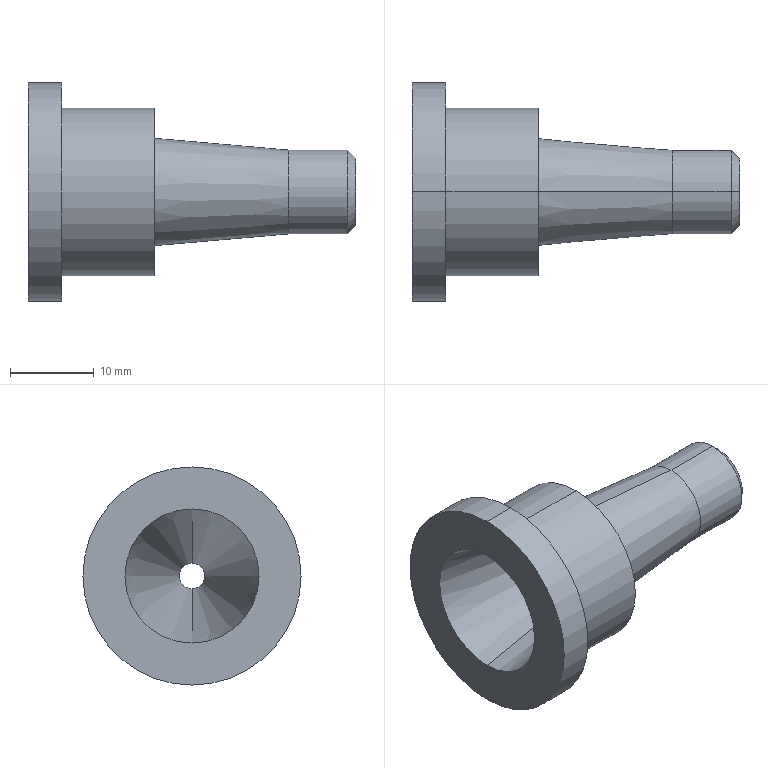Part | SolidWorks | features Chamfer 1, Extrusion 1, RevCut 1, Revolution 1 | 1 solid | 18 faces | box 39 x 26 x 26 mm | volume 5238 mm3 | cylinder 8 | cone 6 | plane 4 | commonest cylinder face diameters 3 x2 10 x2 20 x2 26 x2
STEP:
#1=CARTESIAN_POINT('',(39.,0.,-4.));
#2=VERTEX_POINT('',#1);
#3=CARTESIAN_POINT('',(39.,0.,4.));
#4=VERTEX_POINT('',#3);
#5=CARTESIAN_POINT('',(39.,0.,0.));
#6=DIRECTION('',(1.,0.,0.));
#7=DIRECTION('',(0.,0.,1.));
#8=AXIS2_PLACEMENT_3D('',#5,#6,#7);
#9=CIRCLE('',#8,4.);
#10=EDGE_CURVE('',#2,#4,#9,.T.);
#11=ORIENTED_EDGE('',*,*,#10,.F.);
#12=CARTESIAN_POINT('',(38.,0.,-5.));
#13=VERTEX_POINT('',#12);
#14=CARTESIAN_POINT('',(38.,0.,-5.));
#15=DIRECTION('',(-0.7071,0.,-0.7071));
#16=VECTOR('',#15,1000.);
#17=LINE('',#14,#16);
#18=EDGE_CURVE('',#2,#13,#17,.T.);
#19=ORIENTED_EDGE('',*,*,#18,.T.);
#20=CARTESIAN_POINT('',(38.,0.,5.));
#21=VERTEX_POINT('',#20);
#22=CARTESIAN_POINT('',(38.,0.,0.));
#23=DIRECTION('',(-1.,0.,0.));
#24=DIRECTION('',(0.,0.,1.));
#25=AXIS2_PLACEMENT_3D('',#22,#23,#24);
#26=CIRCLE('',#25,5.);
#27=EDGE_CURVE('',#21,#13,#26,.T.);
#28=ORIENTED_EDGE('',*,*,#27,.F.);
#29=CARTESIAN_POINT('',(38.,0.,5.));
#30=DIRECTION('',(-0.7071,0.,0.7071));
#31=VECTOR('',#30,1000.);
#32=LINE('',#29,#31);
#33=EDGE_CURVE('',#4,#21,#32,.T.);
#34=ORIENTED_EDGE('',*,*,#33,.F.);
#35=EDGE_LOOP('',(#11,#19,#28,#34));
#36=FACE_OUTER_BOUND('',#35,.T.);
#37=CARTESIAN_POINT('',(38.,0.,0.));
#38=DIRECTION('',(-1.,0.,0.));
#39=DIRECTION('',(0.,0.,1.));
#40=AXIS2_PLACEMENT_3D('',#37,#38,#39);
#41=CONICAL_SURFACE('',#40,5.,0.7854);
#42=ADVANCED_FACE('',(#36),#41,.T.);
#43=CARTESIAN_POINT('',(39.,0.,-1.5));
#44=VERTEX_POINT('',#43);
#45=CARTESIAN_POINT('',(39.,0.,1.5));
#46=VERTEX_POINT('',#45);
#47=CARTESIAN_POINT('',(39.,0.,0.));
#48=DIRECTION('',(-1.,0.,0.));
#49=DIRECTION('',(0.,0.,1.));
#50=AXIS2_PLACEMENT_3D('',#47,#48,#49);
#51=CIRCLE('',#50,1.5);
#52=EDGE_CURVE('',#44,#46,#51,.T.);
#53=ORIENTED_EDGE('',*,*,#52,.F.);
#54=CARTESIAN_POINT('',(31.,0.,-1.5));
#55=VERTEX_POINT('',#54);
#56=CARTESIAN_POINT('',(0.,0.,-1.5));
#57=DIRECTION('',(-1.,0.,0.));
#58=VECTOR('',#57,1000.);
#59=LINE('',#56,#58);
#60=EDGE_CURVE('',#44,#55,#59,.T.);
#61=ORIENTED_EDGE('',*,*,#60,.T.);
#62=CARTESIAN_POINT('',(31.,0.,1.5));
#63=VERTEX_POINT('',#62);
#64=CARTESIAN_POINT('',(31.,0.,0.));
#65=DIRECTION('',(-1.,0.,0.));
#66=DIRECTION('',(0.,0.,1.));
#67=AXIS2_PLACEMENT_3D('',#64,#65,#66);
#68=CIRCLE('',#67,1.5);
#69=EDGE_CURVE('',#55,#63,#68,.T.);
#70=ORIENTED_EDGE('',*,*,#69,.T.);
#71=CARTESIAN_POINT('',(0.,0.,1.5));
#72=DIRECTION('',(-1.,0.,0.));
#73=VECTOR('',#72,1000.);
#74=LINE('',#71,#73);
#75=EDGE_CURVE('',#46,#63,#74,.T.);
#76=ORIENTED_EDGE('',*,*,#75,.F.);
#77=EDGE_LOOP('',(#53,#61,#70,#76));
#78=FACE_OUTER_BOUND('',#77,.T.);
#79=CARTESIAN_POINT('',(0.,0.,0.));
#80=DIRECTION('',(-1.,0.,0.));
#81=DIRECTION('',(0.,0.,1.));
#82=AXIS2_PLACEMENT_3D('',#79,#80,#81);
#83=CYLINDRICAL_SURFACE('',#82,1.5);
#84=ADVANCED_FACE('',(#78),#83,.F.);
#85=ORIENTED_EDGE('',*,*,#69,.F.);
#86=CARTESIAN_POINT('',(0.,0.,-8.));
#87=VERTEX_POINT('',#86);
#88=CARTESIAN_POINT('',(31.,0.,-1.5));
#89=DIRECTION('',(-0.9787,0.,-0.2052));
#90=VECTOR('',#89,1000.);
#91=LINE('',#88,#90);
#92=EDGE_CURVE('',#55,#87,#91,.T.);
#93=ORIENTED_EDGE('',*,*,#92,.T.);
#94=CARTESIAN_POINT('',(0.,0.,8.));
#95=VERTEX_POINT('',#94);
#96=CARTESIAN_POINT('',(0.,0.,0.));
#97=DIRECTION('',(-1.,0.,0.));
#98=DIRECTION('',(0.,0.,1.));
#99=AXIS2_PLACEMENT_3D('',#96,#97,#98);
#100=CIRCLE('',#99,8.);
#101=EDGE_CURVE('',#87,#95,#100,.T.);
#102=ORIENTED_EDGE('',*,*,#101,.T.);
#103=CARTESIAN_POINT('',(31.,0.,1.5));
#104=DIRECTION('',(-0.9787,0.,0.2052));
#105=VECTOR('',#104,1000.);
#106=LINE('',#103,#105);
#107=EDGE_CURVE('',#63,#95,#106,.T.);
#108=ORIENTED_EDGE('',*,*,#107,.F.);
#109=EDGE_LOOP('',(#85,#93,#102,#108));
#110=FACE_OUTER_BOUND('',#109,.T.);
#111=CARTESIAN_POINT('',(31.,0.,0.));
#112=DIRECTION('',(-1.,0.,0.));
#113=DIRECTION('',(0.,0.,1.));
#114=AXIS2_PLACEMENT_3D('',#111,#112,#113);
#115=CONICAL_SURFACE('',#114,1.5,0.2067);
#116=ADVANCED_FACE('',(#110),#115,.F.);
#117=ORIENTED_EDGE('',*,*,#27,.T.);
#118=CARTESIAN_POINT('',(31.,0.,-5.));
#119=VERTEX_POINT('',#118);
#120=CARTESIAN_POINT('',(0.,0.,-5.));
#121=DIRECTION('',(-1.,0.,0.));
#122=VECTOR('',#121,1000.);
#123=LINE('',#120,#122);
#124=EDGE_CURVE('',#13,#119,#123,.T.);
#125=ORIENTED_EDGE('',*,*,#124,.T.);
#126=CARTESIAN_POINT('',(31.,0.,5.));
#127=VERTEX_POINT('',#126);
#128=CARTESIAN_POINT('',(31.,0.,0.));
#129=DIRECTION('',(-1.,0.,0.));
#130=DIRECTION('',(0.,0.,1.));
#131=AXIS2_PLACEMENT_3D('',#128,#129,#130);
#132=CIRCLE('',#131,5.);
#133=EDGE_CURVE('',#127,#119,#132,.T.);
#134=ORIENTED_EDGE('',*,*,#133,.F.);
#135=CARTESIAN_POINT('',(0.,0.,5.));
#136=DIRECTION('',(-1.,0.,0.));
#137=VECTOR('',#136,1000.);
#138=LINE('',#135,#137);
#139=EDGE_CURVE('',#21,#127,#138,.T.);
#140=ORIENTED_EDGE('',*,*,#139,.F.);
#141=EDGE_LOOP('',(#117,#125,#134,#140));
#142=FACE_OUTER_BOUND('',#141,.T.);
#143=CARTESIAN_POINT('',(0.,0.,0.));
#144=DIRECTION('',(-1.,0.,0.));
#145=DIRECTION('',(0.,0.,1.));
#146=AXIS2_PLACEMENT_3D('',#143,#144,#145);
#147=CYLINDRICAL_SURFACE('',#146,5.);
#148=ADVANCED_FACE('',(#142),#147,.T.);
#149=ORIENTED_EDGE('',*,*,#133,.T.);
#150=CARTESIAN_POINT('',(15.,0.,-6.4));
#151=VERTEX_POINT('',#150);
#152=CARTESIAN_POINT('',(31.,0.,-5.));
#153=DIRECTION('',(-0.9962,0.,-0.08716));
#154=VECTOR('',#153,1000.);
#155=LINE('',#152,#154);
#156=EDGE_CURVE('',#119,#151,#155,.T.);
#157=ORIENTED_EDGE('',*,*,#156,.T.);
#158=CARTESIAN_POINT('',(15.,0.,6.4));
#159=VERTEX_POINT('',#158);
#160=CARTESIAN_POINT('',(15.,0.,0.));
#161=DIRECTION('',(-1.,0.,0.));
#162=DIRECTION('',(0.,0.,1.));
#163=AXIS2_PLACEMENT_3D('',#160,#161,#162);
#164=CIRCLE('',#163,6.4);
#165=EDGE_CURVE('',#159,#151,#164,.T.);
#166=ORIENTED_EDGE('',*,*,#165,.F.);
#167=CARTESIAN_POINT('',(31.,0.,5.));
#168=DIRECTION('',(-0.9962,0.,0.08716));
#169=VECTOR('',#168,1000.);
#170=LINE('',#167,#169);
#171=EDGE_CURVE('',#127,#159,#170,.T.);
#172=ORIENTED_EDGE('',*,*,#171,.F.);
#173=EDGE_LOOP('',(#149,#157,#166,#172));
#174=FACE_OUTER_BOUND('',#173,.T.);
#175=CARTESIAN_POINT('',(31.,0.,0.));
#176=DIRECTION('',(-1.,0.,0.));
#177=DIRECTION('',(0.,0.,1.));
#178=AXIS2_PLACEMENT_3D('',#175,#176,#177);
#179=CONICAL_SURFACE('',#178,5.,0.08727);
#180=ADVANCED_FACE('',(#174),#179,.T.);
#181=CARTESIAN_POINT('',(15.,0.,10.));
#182=VERTEX_POINT('',#181);
#183=CARTESIAN_POINT('',(15.,0.,-10.));
#184=VERTEX_POINT('',#183);
#185=CARTESIAN_POINT('',(15.,0.,0.));
#186=DIRECTION('',(-1.,0.,0.));
#187=DIRECTION('',(0.,0.,1.));
#188=AXIS2_PLACEMENT_3D('',#185,#186,#187);
#189=CIRCLE('',#188,10.);
#190=EDGE_CURVE('',#182,#184,#189,.T.);
#191=ORIENTED_EDGE('',*,*,#190,.T.);
#192=CARTESIAN_POINT('',(4.,0.,-10.));
#193=VERTEX_POINT('',#192);
#194=CARTESIAN_POINT('',(0.,0.,-10.));
#195=DIRECTION('',(-1.,0.,0.));
#196=VECTOR('',#195,1000.);
#197=LINE('',#194,#196);
#198=EDGE_CURVE('',#184,#193,#197,.T.);
#199=ORIENTED_EDGE('',*,*,#198,.T.);
#200=CARTESIAN_POINT('',(4.,0.,10.));
#201=VERTEX_POINT('',#200);
#202=CARTESIAN_POINT('',(4.,0.,0.));
#203=DIRECTION('',(-1.,0.,0.));
#204=DIRECTION('',(0.,0.,1.));
#205=AXIS2_PLACEMENT_3D('',#202,#203,#204);
#206=CIRCLE('',#205,10.);
#207=EDGE_CURVE('',#201,#193,#206,.T.);
#208=ORIENTED_EDGE('',*,*,#207,.F.);
#209=CARTESIAN_POINT('',(0.,0.,10.));
#210=DIRECTION('',(-1.,0.,0.));
#211=VECTOR('',#210,1000.);
#212=LINE('',#209,#211);
#213=EDGE_CURVE('',#182,#201,#212,.T.);
#214=ORIENTED_EDGE('',*,*,#213,.F.);
#215=EDGE_LOOP('',(#191,#199,#208,#214));
#216=FACE_OUTER_BOUND('',#215,.T.);
#217=CARTESIAN_POINT('',(0.,0.,0.));
#218=DIRECTION('',(-1.,0.,0.));
#219=DIRECTION('',(0.,0.,1.));
#220=AXIS2_PLACEMENT_3D('',#217,#218,#219);
#221=CYLINDRICAL_SURFACE('',#220,10.);
#222=ADVANCED_FACE('',(#216),#221,.T.);
#223=CARTESIAN_POINT('',(4.,0.,13.));
#224=VERTEX_POINT('',#223);
#225=CARTESIAN_POINT('',(4.,0.,-13.));
#226=VERTEX_POINT('',#225);
#227=CARTESIAN_POINT('',(4.,0.,0.));
#228=DIRECTION('',(-1.,0.,0.));
#229=DIRECTION('',(0.,0.,1.));
#230=AXIS2_PLACEMENT_3D('',#227,#228,#229);
#231=CIRCLE('',#230,13.);
#232=EDGE_CURVE('',#224,#226,#231,.T.);
#233=ORIENTED_EDGE('',*,*,#232,.T.);
#234=CARTESIAN_POINT('',(0.,0.,-13.));
#235=VERTEX_POINT('',#234);
#236=CARTESIAN_POINT('',(0.,0.,-13.));
#237=DIRECTION('',(-1.,0.,0.));
#238=VECTOR('',#237,1000.);
#239=LINE('',#236,#238);
#240=EDGE_CURVE('',#226,#235,#239,.T.);
#241=ORIENTED_EDGE('',*,*,#240,.T.);
#242=CARTESIAN_POINT('',(0.,0.,13.));
#243=VERTEX_POINT('',#242);
#244=CARTESIAN_POINT('',(0.,0.,0.));
#245=DIRECTION('',(-1.,0.,0.));
#246=DIRECTION('',(0.,0.,1.));
#247=AXIS2_PLACEMENT_3D('',#244,#245,#246);
#248=CIRCLE('',#247,13.);
#249=EDGE_CURVE('',#243,#235,#248,.T.);
#250=ORIENTED_EDGE('',*,*,#249,.F.);
#251=CARTESIAN_POINT('',(0.,0.,13.));
#252=DIRECTION('',(-1.,0.,0.));
#253=VECTOR('',#252,1000.);
#254=LINE('',#251,#253);
#255=EDGE_CURVE('',#224,#243,#254,.T.);
#256=ORIENTED_EDGE('',*,*,#255,.F.);
#257=EDGE_LOOP('',(#233,#241,#250,#256));
#258=FACE_OUTER_BOUND('',#257,.T.);
#259=CARTESIAN_POINT('',(0.,0.,0.));
#260=DIRECTION('',(-1.,0.,0.));
#261=DIRECTION('',(0.,0.,1.));
#262=AXIS2_PLACEMENT_3D('',#259,#260,#261);
#263=CYLINDRICAL_SURFACE('',#262,13.);
#264=ADVANCED_FACE('',(#258),#263,.T.);
#265=CARTESIAN_POINT('',(0.,0.,0.));
#266=DIRECTION('',(-1.,0.,0.));
#267=DIRECTION('',(0.,0.,1.));
#268=AXIS2_PLACEMENT_3D('',#265,#266,#267);
#269=CIRCLE('',#268,8.);
#270=EDGE_CURVE('',#95,#87,#269,.T.);
#271=ORIENTED_EDGE('',*,*,#270,.F.);
#272=ORIENTED_EDGE('',*,*,#101,.F.);
#273=EDGE_LOOP('',(#271,#272));
#274=FACE_BOUND('',#273,.T.);
#275=ORIENTED_EDGE('',*,*,#249,.T.);
#276=CARTESIAN_POINT('',(0.,0.,0.));
#277=DIRECTION('',(-1.,0.,0.));
#278=DIRECTION('',(0.,0.,1.));
#279=AXIS2_PLACEMENT_3D('',#276,#277,#278);
#280=CIRCLE('',#279,13.);
#281=EDGE_CURVE('',#235,#243,#280,.T.);
#282=ORIENTED_EDGE('',*,*,#281,.T.);
#283=EDGE_LOOP('',(#275,#282));
#284=FACE_OUTER_BOUND('',#283,.T.);
#285=CARTESIAN_POINT('',(0.,0.,0.));
#286=DIRECTION('',(1.,0.,0.));
#287=DIRECTION('',(0.,0.,-1.));
#288=AXIS2_PLACEMENT_3D('',#285,#286,#287);
#289=PLANE('',#288);
#290=ADVANCED_FACE('',(#274,#284),#289,.F.);
#291=ORIENTED_EDGE('',*,*,#240,.F.);
#292=CARTESIAN_POINT('',(4.,0.,0.));
#293=DIRECTION('',(-1.,0.,0.));
#294=DIRECTION('',(0.,0.,1.));
#295=AXIS2_PLACEMENT_3D('',#292,#293,#294);
#296=CIRCLE('',#295,13.);
#297=EDGE_CURVE('',#226,#224,#296,.T.);
#298=ORIENTED_EDGE('',*,*,#297,.T.);
#299=ORIENTED_EDGE('',*,*,#255,.T.);
#300=ORIENTED_EDGE('',*,*,#281,.F.);
#301=EDGE_LOOP('',(#291,#298,#299,#300));
#302=FACE_OUTER_BOUND('',#301,.T.);
#303=CARTESIAN_POINT('',(0.,0.,0.));
#304=DIRECTION('',(-1.,0.,0.));
#305=DIRECTION('',(0.,0.,1.));
#306=AXIS2_PLACEMENT_3D('',#303,#304,#305);
#307=CYLINDRICAL_SURFACE('',#306,13.);
#308=ADVANCED_FACE('',(#302),#307,.T.);
#309=ORIENTED_EDGE('',*,*,#232,.F.);
#310=ORIENTED_EDGE('',*,*,#297,.F.);
#311=EDGE_LOOP('',(#309,#310));
#312=FACE_OUTER_BOUND('',#311,.T.);
#313=ORIENTED_EDGE('',*,*,#207,.T.);
#314=CARTESIAN_POINT('',(4.,0.,0.));
#315=DIRECTION('',(-1.,0.,0.));
#316=DIRECTION('',(0.,0.,1.));
#317=AXIS2_PLACEMENT_3D('',#314,#315,#316);
#318=CIRCLE('',#317,10.);
#319=EDGE_CURVE('',#193,#201,#318,.T.);
#320=ORIENTED_EDGE('',*,*,#319,.T.);
#321=EDGE_LOOP('',(#313,#320));
#322=FACE_BOUND('',#321,.T.);
#323=CARTESIAN_POINT('',(4.,0.,-13.));
#324=DIRECTION('',(-1.,0.,0.));
#325=DIRECTION('',(0.,0.,1.));
#326=AXIS2_PLACEMENT_3D('',#323,#324,#325);
#327=PLANE('',#326);
#328=ADVANCED_FACE('',(#312,#322),#327,.F.);
#329=ORIENTED_EDGE('',*,*,#198,.F.);
#330=CARTESIAN_POINT('',(15.,0.,0.));
#331=DIRECTION('',(-1.,0.,0.));
#332=DIRECTION('',(0.,0.,1.));
#333=AXIS2_PLACEMENT_3D('',#330,#331,#332);
#334=CIRCLE('',#333,10.);
#335=EDGE_CURVE('',#184,#182,#334,.T.);
#336=ORIENTED_EDGE('',*,*,#335,.T.);
#337=ORIENTED_EDGE('',*,*,#213,.T.);
#338=ORIENTED_EDGE('',*,*,#319,.F.);
#339=EDGE_LOOP('',(#329,#336,#337,#338));
#340=FACE_OUTER_BOUND('',#339,.T.);
#341=CARTESIAN_POINT('',(0.,0.,0.));
#342=DIRECTION('',(-1.,0.,0.));
#343=DIRECTION('',(0.,0.,1.));
#344=AXIS2_PLACEMENT_3D('',#341,#342,#343);
#345=CYLINDRICAL_SURFACE('',#344,10.);
#346=ADVANCED_FACE('',(#340),#345,.T.);
#347=ORIENTED_EDGE('',*,*,#190,.F.);
#348=ORIENTED_EDGE('',*,*,#335,.F.);
#349=EDGE_LOOP('',(#347,#348));
#350=FACE_OUTER_BOUND('',#349,.T.);
#351=ORIENTED_EDGE('',*,*,#165,.T.);
#352=CARTESIAN_POINT('',(15.,0.,0.));
#353=DIRECTION('',(-1.,0.,0.));
#354=DIRECTION('',(0.,0.,1.));
#355=AXIS2_PLACEMENT_3D('',#352,#353,#354);
#356=CIRCLE('',#355,6.4);
#357=EDGE_CURVE('',#151,#159,#356,.T.);
#358=ORIENTED_EDGE('',*,*,#357,.T.);
#359=EDGE_LOOP('',(#351,#358));
#360=FACE_BOUND('',#359,.T.);
#361=CARTESIAN_POINT('',(15.,0.,-10.));
#362=DIRECTION('',(-1.,0.,0.));
#363=DIRECTION('',(0.,0.,1.));
#364=AXIS2_PLACEMENT_3D('',#361,#362,#363);
#365=PLANE('',#364);
#366=ADVANCED_FACE('',(#350,#360),#365,.F.);
#367=ORIENTED_EDGE('',*,*,#156,.F.);
#368=CARTESIAN_POINT('',(31.,0.,0.));
#369=DIRECTION('',(-1.,0.,0.));
#370=DIRECTION('',(0.,0.,1.));
#371=AXIS2_PLACEMENT_3D('',#368,#369,#370);
#372=CIRCLE('',#371,5.);
#373=EDGE_CURVE('',#119,#127,#372,.T.);
#374=ORIENTED_EDGE('',*,*,#373,.T.);
#375=ORIENTED_EDGE('',*,*,#171,.T.);
#376=ORIENTED_EDGE('',*,*,#357,.F.);
#377=EDGE_LOOP('',(#367,#374,#375,#376));
#378=FACE_OUTER_BOUND('',#377,.T.);
#379=CARTESIAN_POINT('',(31.,0.,0.));
#380=DIRECTION('',(-1.,0.,0.));
#381=DIRECTION('',(0.,0.,1.));
#382=AXIS2_PLACEMENT_3D('',#379,#380,#381);
#383=CONICAL_SURFACE('',#382,5.,0.08727);
#384=ADVANCED_FACE('',(#378),#383,.T.);
#385=ORIENTED_EDGE('',*,*,#124,.F.);
#386=CARTESIAN_POINT('',(38.,0.,0.));
#387=DIRECTION('',(-1.,0.,0.));
#388=DIRECTION('',(0.,0.,1.));
#389=AXIS2_PLACEMENT_3D('',#386,#387,#388);
#390=CIRCLE('',#389,5.);
#391=EDGE_CURVE('',#13,#21,#390,.T.);
#392=ORIENTED_EDGE('',*,*,#391,.T.);
#393=ORIENTED_EDGE('',*,*,#139,.T.);
#394=ORIENTED_EDGE('',*,*,#373,.F.);
#395=EDGE_LOOP('',(#385,#392,#393,#394));
#396=FACE_OUTER_BOUND('',#395,.T.);
#397=CARTESIAN_POINT('',(0.,0.,0.));
#398=DIRECTION('',(-1.,0.,0.));
#399=DIRECTION('',(0.,0.,1.));
#400=AXIS2_PLACEMENT_3D('',#397,#398,#399);
#401=CYLINDRICAL_SURFACE('',#400,5.);
#402=ADVANCED_FACE('',(#396),#401,.T.);
#403=CARTESIAN_POINT('',(39.,0.,0.));
#404=DIRECTION('',(1.,0.,0.));
#405=DIRECTION('',(0.,0.,1.));
#406=AXIS2_PLACEMENT_3D('',#403,#404,#405);
#407=CIRCLE('',#406,4.);
#408=EDGE_CURVE('',#4,#2,#407,.T.);
#409=ORIENTED_EDGE('',*,*,#408,.T.);
#410=ORIENTED_EDGE('',*,*,#10,.T.);
#411=EDGE_LOOP('',(#409,#410));
#412=FACE_OUTER_BOUND('',#411,.T.);
#413=CARTESIAN_POINT('',(39.,0.,0.));
#414=DIRECTION('',(-1.,0.,0.));
#415=DIRECTION('',(0.,0.,1.));
#416=AXIS2_PLACEMENT_3D('',#413,#414,#415);
#417=CIRCLE('',#416,1.5);
#418=EDGE_CURVE('',#46,#44,#417,.T.);
#419=ORIENTED_EDGE('',*,*,#418,.T.);
#420=ORIENTED_EDGE('',*,*,#52,.T.);
#421=EDGE_LOOP('',(#419,#420));
#422=FACE_BOUND('',#421,.T.);
#423=CARTESIAN_POINT('',(39.,0.,-5.));
#424=DIRECTION('',(-1.,0.,0.));
#425=DIRECTION('',(0.,0.,1.));
#426=AXIS2_PLACEMENT_3D('',#423,#424,#425);
#427=PLANE('',#426);
#428=ADVANCED_FACE('',(#412,#422),#427,.F.);
#429=ORIENTED_EDGE('',*,*,#92,.F.);
#430=CARTESIAN_POINT('',(31.,0.,0.));
#431=DIRECTION('',(-1.,0.,0.));
#432=DIRECTION('',(0.,0.,1.));
#433=AXIS2_PLACEMENT_3D('',#430,#431,#432);
#434=CIRCLE('',#433,1.5);
#435=EDGE_CURVE('',#63,#55,#434,.T.);
#436=ORIENTED_EDGE('',*,*,#435,.F.);
#437=ORIENTED_EDGE('',*,*,#107,.T.);
#438=ORIENTED_EDGE('',*,*,#270,.T.);
#439=EDGE_LOOP('',(#429,#436,#437,#438));
#440=FACE_OUTER_BOUND('',#439,.T.);
#441=CARTESIAN_POINT('',(31.,0.,0.));
#442=DIRECTION('',(-1.,0.,0.));
#443=DIRECTION('',(0.,0.,1.));
#444=AXIS2_PLACEMENT_3D('',#441,#442,#443);
#445=CONICAL_SURFACE('',#444,1.5,0.2067);
#446=ADVANCED_FACE('',(#440),#445,.F.);
#447=ORIENTED_EDGE('',*,*,#60,.F.);
#448=ORIENTED_EDGE('',*,*,#418,.F.);
#449=ORIENTED_EDGE('',*,*,#75,.T.);
#450=ORIENTED_EDGE('',*,*,#435,.T.);
#451=EDGE_LOOP('',(#447,#448,#449,#450));
#452=FACE_OUTER_BOUND('',#451,.T.);
#453=CARTESIAN_POINT('',(0.,0.,0.));
#454=DIRECTION('',(-1.,0.,0.));
#455=DIRECTION('',(0.,0.,1.));
#456=AXIS2_PLACEMENT_3D('',#453,#454,#455);
#457=CYLINDRICAL_SURFACE('',#456,1.5);
#458=ADVANCED_FACE('',(#452),#457,.F.);
#459=ORIENTED_EDGE('',*,*,#18,.F.);
#460=ORIENTED_EDGE('',*,*,#408,.F.);
#461=ORIENTED_EDGE('',*,*,#33,.T.);
#462=ORIENTED_EDGE('',*,*,#391,.F.);
#463=EDGE_LOOP('',(#459,#460,#461,#462));
#464=FACE_OUTER_BOUND('',#463,.T.);
#465=CARTESIAN_POINT('',(38.,0.,0.));
#466=DIRECTION('',(-1.,0.,0.));
#467=DIRECTION('',(0.,0.,1.));
#468=AXIS2_PLACEMENT_3D('',#465,#466,#467);
#469=CONICAL_SURFACE('',#468,5.,0.7854);
#470=ADVANCED_FACE('',(#464),#469,.T.);
#471=CLOSED_SHELL('',(#42,#84,#116,#148,#180,#222,#264,#290,#308,#328,#346,#366,#384,#402,#428,#446,#458,#470));
#472=MANIFOLD_SOLID_BREP('',#471);
#473=CARTESIAN_POINT('',(0.,0.,0.));
#474=DIRECTION('',(0.,0.,1.));
#475=DIRECTION('',(1.,0.,0.));
#476=AXIS2_PLACEMENT_3D('',#473,#474,#475);
#477=(LENGTH_UNIT()NAMED_UNIT(*)SI_UNIT(.MILLI.,.METRE.));
#478=UNCERTAINTY_MEASURE_WITH_UNIT(LENGTH_MEASURE(0.00001),#477,'','');
#479=(NAMED_UNIT(*)PLANE_ANGLE_UNIT()SI_UNIT($,.RADIAN.));
#480=(NAMED_UNIT(*)SI_UNIT($,.STERADIAN.)SOLID_ANGLE_UNIT());
#481=(GEOMETRIC_REPRESENTATION_CONTEXT(3)GLOBAL_UNCERTAINTY_ASSIGNED_CONTEXT((#478))GLOBAL_UNIT_ASSIGNED_CONTEXT((#477,#479,#480))REPRESENTATION_CONTEXT('',''));
#482=ADVANCED_BREP_SHAPE_REPRESENTATION('',(#472,#476),#481);